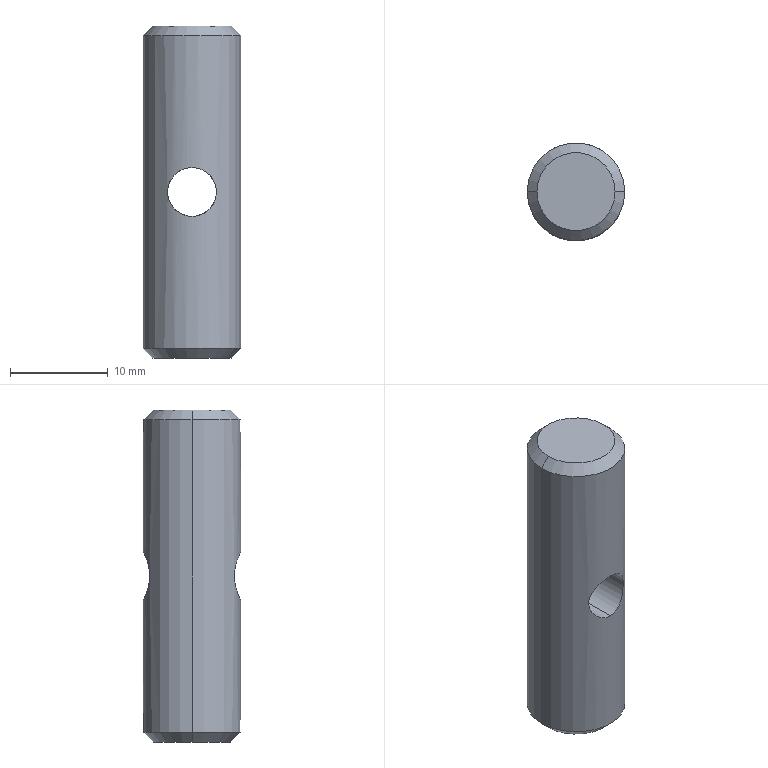Part | SolidWorks | features 3DProfileFeature 1, Chamfer 1, HoleWzd 1, Revolution 1 | 1 solid | 10 faces | box 10 x 10 x 34 mm | volume 2451 mm3 | cone 4 | cylinder 4 | plane 2 | commonest cylinder face diameters 5 x2 10 x2
STEP:
#1=CARTESIAN_POINT('',(-4.,0.,0.));
#2=VERTEX_POINT('',#1);
#3=CARTESIAN_POINT('',(4.,0.,0.));
#4=VERTEX_POINT('',#3);
#5=CARTESIAN_POINT('',(0.,0.,0.));
#6=DIRECTION('',(0.,0.,-1.));
#7=DIRECTION('',(-1.,0.,0.));
#8=AXIS2_PLACEMENT_3D('',#5,#6,#7);
#9=CIRCLE('',#8,4.);
#10=EDGE_CURVE('',#2,#4,#9,.T.);
#11=ORIENTED_EDGE('',*,*,#10,.F.);
#12=CARTESIAN_POINT('',(-5.,0.,1.));
#13=VERTEX_POINT('',#12);
#14=CARTESIAN_POINT('',(-4.,0.,0.));
#15=DIRECTION('',(-0.7071,0.,0.7071));
#16=VECTOR('',#15,1000.);
#17=LINE('',#14,#16);
#18=EDGE_CURVE('',#2,#13,#17,.T.);
#19=ORIENTED_EDGE('',*,*,#18,.T.);
#20=CARTESIAN_POINT('',(5.,0.,1.));
#21=VERTEX_POINT('',#20);
#22=CARTESIAN_POINT('',(0.,0.,1.));
#23=DIRECTION('',(0.,0.,1.));
#24=DIRECTION('',(-1.,0.,0.));
#25=AXIS2_PLACEMENT_3D('',#22,#23,#24);
#26=CIRCLE('',#25,5.);
#27=EDGE_CURVE('',#21,#13,#26,.T.);
#28=ORIENTED_EDGE('',*,*,#27,.F.);
#29=CARTESIAN_POINT('',(4.,0.,0.));
#30=DIRECTION('',(0.7071,0.,0.7071));
#31=VECTOR('',#30,1000.);
#32=LINE('',#29,#31);
#33=EDGE_CURVE('',#4,#21,#32,.T.);
#34=ORIENTED_EDGE('',*,*,#33,.F.);
#35=EDGE_LOOP('',(#11,#19,#28,#34));
#36=FACE_OUTER_BOUND('',#35,.T.);
#37=CARTESIAN_POINT('',(0.,0.,0.));
#38=DIRECTION('',(0.,0.,1.));
#39=DIRECTION('',(1.,0.,0.));
#40=AXIS2_PLACEMENT_3D('',#37,#38,#39);
#41=CONICAL_SURFACE('',#40,4.,0.7854);
#42=ADVANCED_FACE('',(#36),#41,.T.);
#43=CARTESIAN_POINT('',(4.,0.,34.));
#44=VERTEX_POINT('',#43);
#45=CARTESIAN_POINT('',(-4.,0.,34.));
#46=VERTEX_POINT('',#45);
#47=CARTESIAN_POINT('',(0.,0.,34.));
#48=DIRECTION('',(0.,0.,1.));
#49=DIRECTION('',(1.,0.,0.));
#50=AXIS2_PLACEMENT_3D('',#47,#48,#49);
#51=CIRCLE('',#50,4.);
#52=EDGE_CURVE('',#44,#46,#51,.T.);
#53=ORIENTED_EDGE('',*,*,#52,.F.);
#54=CARTESIAN_POINT('',(5.,0.,33.));
#55=VERTEX_POINT('',#54);
#56=CARTESIAN_POINT('',(5.,0.,33.));
#57=DIRECTION('',(0.7071,0.,-0.7071));
#58=VECTOR('',#57,1000.);
#59=LINE('',#56,#58);
#60=EDGE_CURVE('',#44,#55,#59,.T.);
#61=ORIENTED_EDGE('',*,*,#60,.T.);
#62=CARTESIAN_POINT('',(-5.,0.,33.));
#63=VERTEX_POINT('',#62);
#64=CARTESIAN_POINT('',(0.,0.,33.));
#65=DIRECTION('',(0.,0.,-1.));
#66=DIRECTION('',(1.,0.,0.));
#67=AXIS2_PLACEMENT_3D('',#64,#65,#66);
#68=CIRCLE('',#67,5.);
#69=EDGE_CURVE('',#63,#55,#68,.T.);
#70=ORIENTED_EDGE('',*,*,#69,.F.);
#71=CARTESIAN_POINT('',(-5.,0.,33.));
#72=DIRECTION('',(-0.7071,0.,-0.7071));
#73=VECTOR('',#72,1000.);
#74=LINE('',#71,#73);
#75=EDGE_CURVE('',#46,#63,#74,.T.);
#76=ORIENTED_EDGE('',*,*,#75,.F.);
#77=EDGE_LOOP('',(#53,#61,#70,#76));
#78=FACE_OUTER_BOUND('',#77,.T.);
#79=CARTESIAN_POINT('',(0.,0.,33.));
#80=DIRECTION('',(0.,0.,-1.));
#81=DIRECTION('',(-1.,0.,0.));
#82=AXIS2_PLACEMENT_3D('',#79,#80,#81);
#83=CONICAL_SURFACE('',#82,5.,0.7854);
#84=ADVANCED_FACE('',(#78),#83,.T.);
#85=CARTESIAN_POINT('',(0.,5.,14.5));
#86=VERTEX_POINT('',#85);
#87=CARTESIAN_POINT('',(0.,5.,19.5));
#88=VERTEX_POINT('',#87);
#89=CARTESIAN_POINT('',(0.,5.,14.5));
#90=CARTESIAN_POINT('',(-0.1682,5.,14.5));
#91=CARTESIAN_POINT('',(-0.3332,4.992,14.517));
#92=CARTESIAN_POINT('',(-0.6568,4.959,14.582));
#93=CARTESIAN_POINT('',(-0.8171,4.935,14.632));
#94=CARTESIAN_POINT('',(-1.27,4.846,14.822));
#95=CARTESIAN_POINT('',(-1.543,4.762,15.007));
#96=CARTESIAN_POINT('',(-1.883,4.633,15.348));
#97=CARTESIAN_POINT('',(-1.986,4.59,15.473));
#98=CARTESIAN_POINT('',(-2.166,4.507,15.742));
#99=CARTESIAN_POINT('',(-2.243,4.469,15.884));
#100=CARTESIAN_POINT('',(-2.368,4.404,16.183));
#101=CARTESIAN_POINT('',(-2.418,4.377,16.343));
#102=CARTESIAN_POINT('',(-2.483,4.34,16.667));
#103=CARTESIAN_POINT('',(-2.5,4.33,16.831));
#104=CARTESIAN_POINT('',(-2.5,4.33,17.164));
#105=CARTESIAN_POINT('',(-2.483,4.34,17.333));
#106=CARTESIAN_POINT('',(-2.418,4.377,17.656));
#107=CARTESIAN_POINT('',(-2.369,4.404,17.815));
#108=CARTESIAN_POINT('',(-2.242,4.47,18.117));
#109=CARTESIAN_POINT('',(-2.165,4.508,18.26));
#110=CARTESIAN_POINT('',(-1.985,4.59,18.528));
#111=CARTESIAN_POINT('',(-1.881,4.634,18.654));
#112=CARTESIAN_POINT('',(-1.541,4.763,18.994));
#113=CARTESIAN_POINT('',(-1.266,4.847,19.18));
#114=CARTESIAN_POINT('',(-0.8162,4.935,19.369));
#115=CARTESIAN_POINT('',(-0.6575,4.959,19.418));
#116=CARTESIAN_POINT('',(-0.3307,4.992,19.484));
#117=CARTESIAN_POINT('',(-0.166,5.,19.5));
#118=CARTESIAN_POINT('',(0.,5.,19.5));
#119=B_SPLINE_CURVE_WITH_KNOTS('',3,(#89,#90,#91,#92,#93,#94,#95,#96,#97,#98,#99,#100,#101,#102,#103,#104,#105,#106,#107,#108,#109,#110,#111,#112,#113,#114,#115,#116,#117,#118),.UNSPECIFIED.,.F.,.F.,(4,2,2,2,2,2,2,2,2,2,2,2,2,2,4),(0.,0.000497,0.0009941,0.001988,0.002485,0.002982,0.003479,0.003976,0.004473,0.00497,0.005467,0.005964,0.006958,0.007455,0.007952),.UNSPECIFIED.);
#120=EDGE_CURVE('',#86,#88,#119,.T.);
#121=ORIENTED_EDGE('',*,*,#120,.T.);
#122=CARTESIAN_POINT('',(0.,-5.,19.5));
#123=VERTEX_POINT('',#122);
#124=CARTESIAN_POINT('',(0.,-5.,19.5));
#125=DIRECTION('',(0.,-1.,0.));
#126=VECTOR('',#125,1000.);
#127=LINE('',#124,#126);
#128=EDGE_CURVE('',#88,#123,#127,.T.);
#129=ORIENTED_EDGE('',*,*,#128,.T.);
#130=CARTESIAN_POINT('',(0.,-5.,14.5));
#131=VERTEX_POINT('',#130);
#132=CARTESIAN_POINT('',(0.,-5.,19.5));
#133=CARTESIAN_POINT('',(-0.1657,-5.,19.5));
#134=CARTESIAN_POINT('',(-0.3343,-4.991,19.483));
#135=CARTESIAN_POINT('',(-0.6583,-4.959,19.417));
#136=CARTESIAN_POINT('',(-0.8154,-4.936,19.369));
#137=CARTESIAN_POINT('',(-1.12,-4.875,19.241));
#138=CARTESIAN_POINT('',(-1.263,-4.84,19.164));
#139=CARTESIAN_POINT('',(-1.531,-4.762,18.983));
#140=CARTESIAN_POINT('',(-1.657,-4.719,18.879));
#141=CARTESIAN_POINT('',(-1.884,-4.633,18.652));
#142=CARTESIAN_POINT('',(-1.985,-4.59,18.528));
#143=CARTESIAN_POINT('',(-2.165,-4.508,18.26));
#144=CARTESIAN_POINT('',(-2.243,-4.469,18.115));
#145=CARTESIAN_POINT('',(-2.368,-4.404,17.816));
#146=CARTESIAN_POINT('',(-2.417,-4.377,17.661));
#147=CARTESIAN_POINT('',(-2.483,-4.34,17.334));
#148=CARTESIAN_POINT('',(-2.5,-4.33,17.168));
#149=CARTESIAN_POINT('',(-2.5,-4.33,16.837));
#150=CARTESIAN_POINT('',(-2.484,-4.34,16.67));
#151=CARTESIAN_POINT('',(-2.418,-4.377,16.344));
#152=CARTESIAN_POINT('',(-2.37,-4.403,16.188));
#153=CARTESIAN_POINT('',(-2.181,-4.502,15.734));
#154=CARTESIAN_POINT('',(-1.997,-4.59,15.462));
#155=CARTESIAN_POINT('',(-1.655,-4.72,15.12));
#156=CARTESIAN_POINT('',(-1.532,-4.762,15.018));
#157=CARTESIAN_POINT('',(-1.264,-4.84,14.837));
#158=CARTESIAN_POINT('',(-1.119,-4.876,14.758));
#159=CARTESIAN_POINT('',(-0.8175,-4.935,14.632));
#160=CARTESIAN_POINT('',(-0.6613,-4.959,14.583));
#161=CARTESIAN_POINT('',(-0.3368,-4.991,14.517));
#162=CARTESIAN_POINT('',(-0.168,-5.,14.5));
#163=CARTESIAN_POINT('',(0.,-5.,14.5));
#164=B_SPLINE_CURVE_WITH_KNOTS('',3,(#132,#133,#134,#135,#136,#137,#138,#139,#140,#141,#142,#143,#144,#145,#146,#147,#148,#149,#150,#151,#152,#153,#154,#155,#156,#157,#158,#159,#160,#161,#162,#163),.UNSPECIFIED.,.F.,.F.,(4,2,2,2,2,2,2,2,2,2,2,2,2,2,2,4),(0.007952,0.008449,0.008945,0.009441,0.009937,0.01043,0.01093,0.01143,0.01192,0.01242,0.01291,0.01391,0.0144,0.0149,0.01539,0.01589),.UNSPECIFIED.);
#165=EDGE_CURVE('',#123,#131,#164,.T.);
#166=ORIENTED_EDGE('',*,*,#165,.T.);
#167=CARTESIAN_POINT('',(0.,-5.,14.5));
#168=DIRECTION('',(0.,-1.,0.));
#169=VECTOR('',#168,1000.);
#170=LINE('',#167,#169);
#171=EDGE_CURVE('',#86,#131,#170,.T.);
#172=ORIENTED_EDGE('',*,*,#171,.F.);
#173=EDGE_LOOP('',(#121,#129,#166,#172));
#174=FACE_OUTER_BOUND('',#173,.T.);
#175=CARTESIAN_POINT('',(0.,-5.,17.));
#176=DIRECTION('',(0.,-1.,0.));
#177=DIRECTION('',(0.,0.,-1.));
#178=AXIS2_PLACEMENT_3D('',#175,#176,#177);
#179=CYLINDRICAL_SURFACE('',#178,2.5);
#180=ADVANCED_FACE('',(#174),#179,.F.);
#181=ORIENTED_EDGE('',*,*,#120,.F.);
#182=CARTESIAN_POINT('',(0.,5.,19.5));
#183=CARTESIAN_POINT('',(0.1657,5.,19.5));
#184=CARTESIAN_POINT('',(0.3343,4.991,19.483));
#185=CARTESIAN_POINT('',(0.6583,4.959,19.417));
#186=CARTESIAN_POINT('',(0.8154,4.936,19.369));
#187=CARTESIAN_POINT('',(1.12,4.875,19.241));
#188=CARTESIAN_POINT('',(1.263,4.84,19.164));
#189=CARTESIAN_POINT('',(1.531,4.762,18.983));
#190=CARTESIAN_POINT('',(1.657,4.719,18.879));
#191=CARTESIAN_POINT('',(1.884,4.633,18.652));
#192=CARTESIAN_POINT('',(1.985,4.59,18.528));
#193=CARTESIAN_POINT('',(2.165,4.508,18.26));
#194=CARTESIAN_POINT('',(2.243,4.469,18.115));
#195=CARTESIAN_POINT('',(2.368,4.404,17.816));
#196=CARTESIAN_POINT('',(2.417,4.377,17.661));
#197=CARTESIAN_POINT('',(2.483,4.34,17.334));
#198=CARTESIAN_POINT('',(2.5,4.33,17.168));
#199=CARTESIAN_POINT('',(2.5,4.33,16.837));
#200=CARTESIAN_POINT('',(2.484,4.34,16.67));
#201=CARTESIAN_POINT('',(2.418,4.377,16.344));
#202=CARTESIAN_POINT('',(2.37,4.403,16.188));
#203=CARTESIAN_POINT('',(2.181,4.502,15.734));
#204=CARTESIAN_POINT('',(1.997,4.59,15.462));
#205=CARTESIAN_POINT('',(1.655,4.72,15.12));
#206=CARTESIAN_POINT('',(1.532,4.762,15.018));
#207=CARTESIAN_POINT('',(1.264,4.84,14.837));
#208=CARTESIAN_POINT('',(1.119,4.876,14.758));
#209=CARTESIAN_POINT('',(0.8175,4.935,14.632));
#210=CARTESIAN_POINT('',(0.6613,4.959,14.583));
#211=CARTESIAN_POINT('',(0.3368,4.991,14.517));
#212=CARTESIAN_POINT('',(0.168,5.,14.5));
#213=CARTESIAN_POINT('',(0.,5.,14.5));
#214=B_SPLINE_CURVE_WITH_KNOTS('',3,(#182,#183,#184,#185,#186,#187,#188,#189,#190,#191,#192,#193,#194,#195,#196,#197,#198,#199,#200,#201,#202,#203,#204,#205,#206,#207,#208,#209,#210,#211,#212,#213),.UNSPECIFIED.,.F.,.F.,(4,2,2,2,2,2,2,2,2,2,2,2,2,2,2,4),(0.007952,0.008449,0.008945,0.009441,0.009937,0.01043,0.01093,0.01143,0.01192,0.01242,0.01291,0.01391,0.0144,0.0149,0.01539,0.01589),.UNSPECIFIED.);
#215=EDGE_CURVE('',#88,#86,#214,.T.);
#216=ORIENTED_EDGE('',*,*,#215,.F.);
#217=EDGE_LOOP('',(#181,#216));
#218=FACE_BOUND('',#217,.T.);
#219=ORIENTED_EDGE('',*,*,#69,.T.);
#220=CARTESIAN_POINT('',(5.,0.,34.));
#221=DIRECTION('',(0.,0.,-1.));
#222=VECTOR('',#221,1000.);
#223=LINE('',#220,#222);
#224=EDGE_CURVE('',#55,#21,#223,.T.);
#225=ORIENTED_EDGE('',*,*,#224,.T.);
#226=ORIENTED_EDGE('',*,*,#27,.T.);
#227=CARTESIAN_POINT('',(-5.,0.,34.));
#228=DIRECTION('',(0.,0.,-1.));
#229=VECTOR('',#228,1000.);
#230=LINE('',#227,#229);
#231=EDGE_CURVE('',#63,#13,#230,.T.);
#232=ORIENTED_EDGE('',*,*,#231,.F.);
#233=EDGE_LOOP('',(#219,#225,#226,#232));
#234=FACE_OUTER_BOUND('',#233,.T.);
#235=CARTESIAN_POINT('',(0.,0.,34.));
#236=DIRECTION('',(0.,0.,-1.));
#237=DIRECTION('',(-1.,0.,0.));
#238=AXIS2_PLACEMENT_3D('',#235,#236,#237);
#239=CYLINDRICAL_SURFACE('',#238,5.);
#240=ADVANCED_FACE('',(#218,#234),#239,.T.);
#241=ORIENTED_EDGE('',*,*,#224,.F.);
#242=CARTESIAN_POINT('',(0.,0.,33.));
#243=DIRECTION('',(0.,0.,-1.));
#244=DIRECTION('',(1.,0.,0.));
#245=AXIS2_PLACEMENT_3D('',#242,#243,#244);
#246=CIRCLE('',#245,5.);
#247=EDGE_CURVE('',#55,#63,#246,.T.);
#248=ORIENTED_EDGE('',*,*,#247,.T.);
#249=ORIENTED_EDGE('',*,*,#231,.T.);
#250=CARTESIAN_POINT('',(0.,0.,1.));
#251=DIRECTION('',(0.,0.,1.));
#252=DIRECTION('',(-1.,0.,0.));
#253=AXIS2_PLACEMENT_3D('',#250,#251,#252);
#254=CIRCLE('',#253,5.);
#255=EDGE_CURVE('',#13,#21,#254,.T.);
#256=ORIENTED_EDGE('',*,*,#255,.T.);
#257=EDGE_LOOP('',(#241,#248,#249,#256));
#258=FACE_OUTER_BOUND('',#257,.T.);
#259=CARTESIAN_POINT('',(0.,-5.,14.5));
#260=CARTESIAN_POINT('',(0.1682,-5.,14.5));
#261=CARTESIAN_POINT('',(0.3332,-4.992,14.517));
#262=CARTESIAN_POINT('',(0.6568,-4.959,14.582));
#263=CARTESIAN_POINT('',(0.8171,-4.935,14.632));
#264=CARTESIAN_POINT('',(1.27,-4.846,14.822));
#265=CARTESIAN_POINT('',(1.543,-4.762,15.007));
#266=CARTESIAN_POINT('',(1.883,-4.633,15.348));
#267=CARTESIAN_POINT('',(1.986,-4.59,15.473));
#268=CARTESIAN_POINT('',(2.166,-4.507,15.742));
#269=CARTESIAN_POINT('',(2.243,-4.469,15.884));
#270=CARTESIAN_POINT('',(2.368,-4.404,16.183));
#271=CARTESIAN_POINT('',(2.418,-4.377,16.343));
#272=CARTESIAN_POINT('',(2.483,-4.34,16.667));
#273=CARTESIAN_POINT('',(2.5,-4.33,16.831));
#274=CARTESIAN_POINT('',(2.5,-4.33,17.164));
#275=CARTESIAN_POINT('',(2.483,-4.34,17.333));
#276=CARTESIAN_POINT('',(2.418,-4.377,17.656));
#277=CARTESIAN_POINT('',(2.369,-4.404,17.815));
#278=CARTESIAN_POINT('',(2.242,-4.47,18.117));
#279=CARTESIAN_POINT('',(2.165,-4.508,18.26));
#280=CARTESIAN_POINT('',(1.985,-4.59,18.528));
#281=CARTESIAN_POINT('',(1.881,-4.634,18.654));
#282=CARTESIAN_POINT('',(1.541,-4.763,18.994));
#283=CARTESIAN_POINT('',(1.266,-4.847,19.18));
#284=CARTESIAN_POINT('',(0.8162,-4.935,19.369));
#285=CARTESIAN_POINT('',(0.6575,-4.959,19.418));
#286=CARTESIAN_POINT('',(0.3307,-4.992,19.484));
#287=CARTESIAN_POINT('',(0.166,-5.,19.5));
#288=CARTESIAN_POINT('',(0.,-5.,19.5));
#289=B_SPLINE_CURVE_WITH_KNOTS('',3,(#259,#260,#261,#262,#263,#264,#265,#266,#267,#268,#269,#270,#271,#272,#273,#274,#275,#276,#277,#278,#279,#280,#281,#282,#283,#284,#285,#286,#287,#288),.UNSPECIFIED.,.F.,.F.,(4,2,2,2,2,2,2,2,2,2,2,2,2,2,4),(0.,0.000497,0.0009941,0.001988,0.002485,0.002982,0.003479,0.003976,0.004473,0.00497,0.005467,0.005964,0.006958,0.007455,0.007952),.UNSPECIFIED.);
#290=EDGE_CURVE('',#131,#123,#289,.T.);
#291=ORIENTED_EDGE('',*,*,#290,.F.);
#292=ORIENTED_EDGE('',*,*,#165,.F.);
#293=EDGE_LOOP('',(#291,#292));
#294=FACE_BOUND('',#293,.T.);
#295=CARTESIAN_POINT('',(0.,0.,34.));
#296=DIRECTION('',(0.,0.,-1.));
#297=DIRECTION('',(-1.,0.,0.));
#298=AXIS2_PLACEMENT_3D('',#295,#296,#297);
#299=CYLINDRICAL_SURFACE('',#298,5.);
#300=ADVANCED_FACE('',(#258,#294),#299,.T.);
#301=CARTESIAN_POINT('',(0.,0.,34.));
#302=DIRECTION('',(0.,0.,1.));
#303=DIRECTION('',(1.,0.,0.));
#304=AXIS2_PLACEMENT_3D('',#301,#302,#303);
#305=CIRCLE('',#304,4.);
#306=EDGE_CURVE('',#46,#44,#305,.T.);
#307=ORIENTED_EDGE('',*,*,#306,.T.);
#308=ORIENTED_EDGE('',*,*,#52,.T.);
#309=EDGE_LOOP('',(#307,#308));
#310=FACE_OUTER_BOUND('',#309,.T.);
#311=CARTESIAN_POINT('',(5.,0.,34.));
#312=DIRECTION('',(0.,0.,1.));
#313=DIRECTION('',(1.,0.,0.));
#314=AXIS2_PLACEMENT_3D('',#311,#312,#313);
#315=PLANE('',#314);
#316=ADVANCED_FACE('',(#310),#315,.T.);
#317=CARTESIAN_POINT('',(0.,0.,0.));
#318=DIRECTION('',(0.,0.,-1.));
#319=DIRECTION('',(-1.,0.,0.));
#320=AXIS2_PLACEMENT_3D('',#317,#318,#319);
#321=CIRCLE('',#320,4.);
#322=EDGE_CURVE('',#4,#2,#321,.T.);
#323=ORIENTED_EDGE('',*,*,#322,.T.);
#324=ORIENTED_EDGE('',*,*,#10,.T.);
#325=EDGE_LOOP('',(#323,#324));
#326=FACE_OUTER_BOUND('',#325,.T.);
#327=CARTESIAN_POINT('',(0.,0.,0.));
#328=DIRECTION('',(0.,0.,-1.));
#329=DIRECTION('',(-1.,0.,0.));
#330=AXIS2_PLACEMENT_3D('',#327,#328,#329);
#331=PLANE('',#330);
#332=ADVANCED_FACE('',(#326),#331,.T.);
#333=ORIENTED_EDGE('',*,*,#128,.F.);
#334=ORIENTED_EDGE('',*,*,#215,.T.);
#335=ORIENTED_EDGE('',*,*,#171,.T.);
#336=ORIENTED_EDGE('',*,*,#290,.T.);
#337=EDGE_LOOP('',(#333,#334,#335,#336));
#338=FACE_OUTER_BOUND('',#337,.T.);
#339=CARTESIAN_POINT('',(0.,-5.,17.));
#340=DIRECTION('',(0.,-1.,0.));
#341=DIRECTION('',(0.,0.,-1.));
#342=AXIS2_PLACEMENT_3D('',#339,#340,#341);
#343=CYLINDRICAL_SURFACE('',#342,2.5);
#344=ADVANCED_FACE('',(#338),#343,.F.);
#345=ORIENTED_EDGE('',*,*,#60,.F.);
#346=ORIENTED_EDGE('',*,*,#306,.F.);
#347=ORIENTED_EDGE('',*,*,#75,.T.);
#348=ORIENTED_EDGE('',*,*,#247,.F.);
#349=EDGE_LOOP('',(#345,#346,#347,#348));
#350=FACE_OUTER_BOUND('',#349,.T.);
#351=CARTESIAN_POINT('',(0.,0.,33.));
#352=DIRECTION('',(0.,0.,-1.));
#353=DIRECTION('',(-1.,0.,0.));
#354=AXIS2_PLACEMENT_3D('',#351,#352,#353);
#355=CONICAL_SURFACE('',#354,5.,0.7854);
#356=ADVANCED_FACE('',(#350),#355,.T.);
#357=ORIENTED_EDGE('',*,*,#18,.F.);
#358=ORIENTED_EDGE('',*,*,#322,.F.);
#359=ORIENTED_EDGE('',*,*,#33,.T.);
#360=ORIENTED_EDGE('',*,*,#255,.F.);
#361=EDGE_LOOP('',(#357,#358,#359,#360));
#362=FACE_OUTER_BOUND('',#361,.T.);
#363=CARTESIAN_POINT('',(0.,0.,0.));
#364=DIRECTION('',(0.,0.,1.));
#365=DIRECTION('',(1.,0.,0.));
#366=AXIS2_PLACEMENT_3D('',#363,#364,#365);
#367=CONICAL_SURFACE('',#366,4.,0.7854);
#368=ADVANCED_FACE('',(#362),#367,.T.);
#369=CLOSED_SHELL('',(#42,#84,#180,#240,#300,#316,#332,#344,#356,#368));
#370=MANIFOLD_SOLID_BREP('',#369);
#371=CARTESIAN_POINT('',(0.,0.,0.));
#372=DIRECTION('',(0.,0.,1.));
#373=DIRECTION('',(1.,0.,0.));
#374=AXIS2_PLACEMENT_3D('',#371,#372,#373);
#375=(LENGTH_UNIT()NAMED_UNIT(*)SI_UNIT(.MILLI.,.METRE.));
#376=UNCERTAINTY_MEASURE_WITH_UNIT(LENGTH_MEASURE(0.00001),#375,'','');
#377=(NAMED_UNIT(*)PLANE_ANGLE_UNIT()SI_UNIT($,.RADIAN.));
#378=(NAMED_UNIT(*)SI_UNIT($,.STERADIAN.)SOLID_ANGLE_UNIT());
#379=(GEOMETRIC_REPRESENTATION_CONTEXT(3)GLOBAL_UNCERTAINTY_ASSIGNED_CONTEXT((#376))GLOBAL_UNIT_ASSIGNED_CONTEXT((#375,#377,#378))REPRESENTATION_CONTEXT('',''));
#380=ADVANCED_BREP_SHAPE_REPRESENTATION('',(#370,#374),#379);